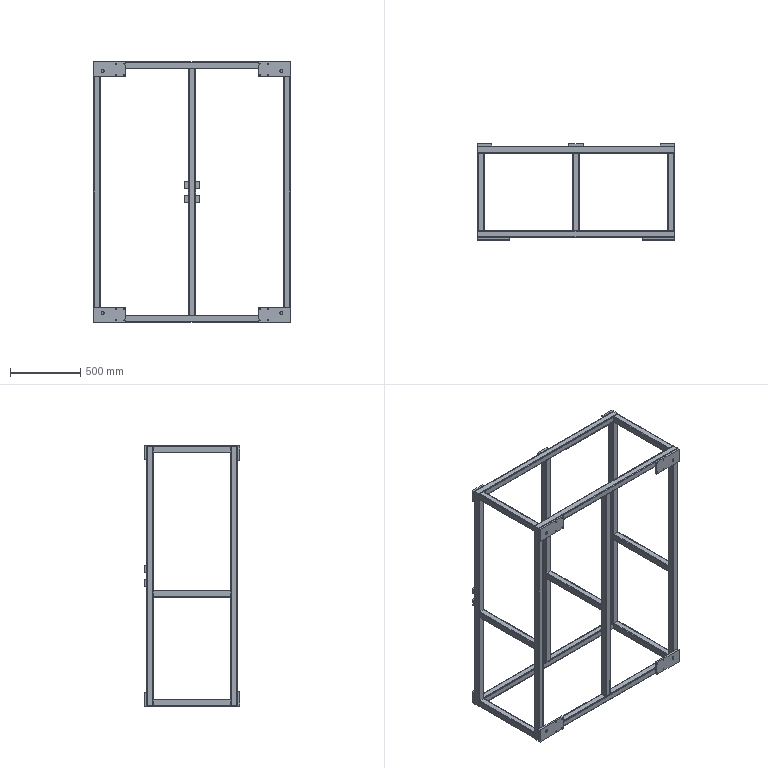Part | SolidWorks | features WeldCornerFeat 8, Chamfer 4, HoleWzd 4, ICE 4, MirrorSolid 4, WeldMemberFeat 4, WeldmentFeature 1 | 33 solids | 668 faces | box 1400 x 680 x 1850 mm | volume 13190709 mm3 | cylinder 292 | plane 288 | cone 88 | commonest cylinder face diameters 12 x120 6.8 x96 6 x68 17.5 x8